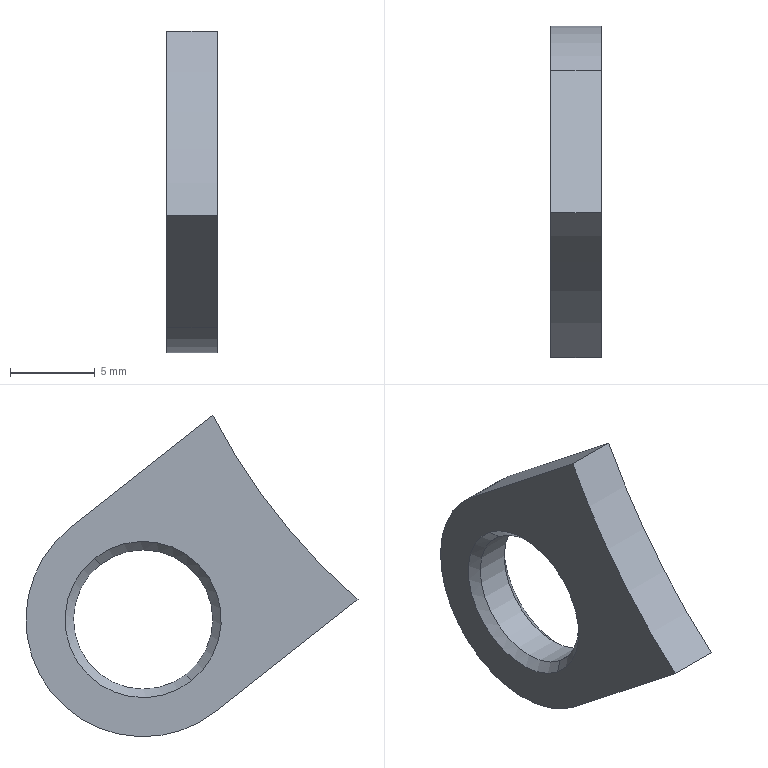Part | SolidWorks | features BaseBody 1 | 1 solid | 12 faces | box 3 x 19.549 x 18.922 mm | volume 482.4 mm3 | cone 4 | cylinder 4 | plane 4 | commonest cylinder face diameters 8.2 x2 13.8 x1 72 x1
STEP:
#1=CARTESIAN_POINT('',(274.5,36.037,-21.279));
#2=VERTEX_POINT('',#1);
#3=CARTESIAN_POINT('',(274.5,30.963,-27.721));
#4=VERTEX_POINT('',#3);
#5=CARTESIAN_POINT('',(274.5,33.5,-24.5));
#6=DIRECTION('',(1.,0.,0.));
#7=DIRECTION('',(0.,-0.6189,-0.7855));
#8=AXIS2_PLACEMENT_3D('',#5,#6,#7);
#9=CIRCLE('',#8,4.1);
#10=EDGE_CURVE('',#2,#4,#9,.T.);
#11=ORIENTED_EDGE('',*,*,#10,.F.);
#12=CARTESIAN_POINT('',(275.,36.347,-20.887));
#13=VERTEX_POINT('',#12);
#14=CARTESIAN_POINT('',(274.5,36.037,-21.279));
#15=DIRECTION('',(0.7071,0.4376,0.5554));
#16=VECTOR('',#15,1000.);
#17=LINE('',#14,#16);
#18=EDGE_CURVE('',#2,#13,#17,.T.);
#19=ORIENTED_EDGE('',*,*,#18,.T.);
#20=CARTESIAN_POINT('',(275.,30.653,-28.113));
#21=VERTEX_POINT('',#20);
#22=CARTESIAN_POINT('',(275.,33.5,-24.5));
#23=DIRECTION('',(-1.,0.,0.));
#24=DIRECTION('',(0.,-0.6189,-0.7855));
#25=AXIS2_PLACEMENT_3D('',#22,#23,#24);
#26=CIRCLE('',#25,4.6);
#27=EDGE_CURVE('',#21,#13,#26,.T.);
#28=ORIENTED_EDGE('',*,*,#27,.F.);
#29=CARTESIAN_POINT('',(274.5,30.963,-27.721));
#30=DIRECTION('',(0.7071,-0.4376,-0.5554));
#31=VECTOR('',#30,1000.);
#32=LINE('',#29,#31);
#33=EDGE_CURVE('',#4,#21,#32,.T.);
#34=ORIENTED_EDGE('',*,*,#33,.F.);
#35=EDGE_LOOP('',(#11,#19,#28,#34));
#36=FACE_OUTER_BOUND('',#35,.T.);
#37=CARTESIAN_POINT('',(274.5,33.5,-24.5));
#38=DIRECTION('',(1.,0.,0.));
#39=DIRECTION('',(0.,-0.6189,-0.7855));
#40=AXIS2_PLACEMENT_3D('',#37,#38,#39);
#41=CONICAL_SURFACE('',#40,4.1,0.7854);
#42=ADVANCED_FACE('',(#36),#41,.F.);
#43=CARTESIAN_POINT('',(272.5,30.963,-27.721));
#44=VERTEX_POINT('',#43);
#45=CARTESIAN_POINT('',(272.5,36.037,-21.279));
#46=VERTEX_POINT('',#45);
#47=CARTESIAN_POINT('',(272.5,33.5,-24.5));
#48=DIRECTION('',(-1.,0.,0.));
#49=DIRECTION('',(0.,-0.6189,-0.7855));
#50=AXIS2_PLACEMENT_3D('',#47,#48,#49);
#51=CIRCLE('',#50,4.1);
#52=EDGE_CURVE('',#44,#46,#51,.T.);
#53=ORIENTED_EDGE('',*,*,#52,.F.);
#54=CARTESIAN_POINT('',(272.,30.653,-28.113));
#55=VERTEX_POINT('',#54);
#56=CARTESIAN_POINT('',(272.,30.653,-28.113));
#57=DIRECTION('',(-0.7071,-0.4376,-0.5554));
#58=VECTOR('',#57,1000.);
#59=LINE('',#56,#58);
#60=EDGE_CURVE('',#44,#55,#59,.T.);
#61=ORIENTED_EDGE('',*,*,#60,.T.);
#62=CARTESIAN_POINT('',(272.,36.347,-20.887));
#63=VERTEX_POINT('',#62);
#64=CARTESIAN_POINT('',(272.,33.5,-24.5));
#65=DIRECTION('',(1.,0.,0.));
#66=DIRECTION('',(0.,-0.6189,-0.7855));
#67=AXIS2_PLACEMENT_3D('',#64,#65,#66);
#68=CIRCLE('',#67,4.6);
#69=EDGE_CURVE('',#63,#55,#68,.T.);
#70=ORIENTED_EDGE('',*,*,#69,.F.);
#71=CARTESIAN_POINT('',(272.,36.347,-20.887));
#72=DIRECTION('',(-0.7071,0.4376,0.5554));
#73=VECTOR('',#72,1000.);
#74=LINE('',#71,#73);
#75=EDGE_CURVE('',#46,#63,#74,.T.);
#76=ORIENTED_EDGE('',*,*,#75,.F.);
#77=EDGE_LOOP('',(#53,#61,#70,#76));
#78=FACE_OUTER_BOUND('',#77,.T.);
#79=CARTESIAN_POINT('',(272.,33.5,-24.5));
#80=DIRECTION('',(-1.,0.,0.));
#81=DIRECTION('',(0.,0.6189,0.7855));
#82=AXIS2_PLACEMENT_3D('',#79,#80,#81);
#83=CONICAL_SURFACE('',#82,4.6,0.7854);
#84=ADVANCED_FACE('',(#78),#83,.F.);
#85=ORIENTED_EDGE('',*,*,#10,.T.);
#86=CARTESIAN_POINT('',(275.,30.963,-27.721));
#87=DIRECTION('',(-1.,0.,0.));
#88=VECTOR('',#87,1000.);
#89=LINE('',#86,#88);
#90=EDGE_CURVE('',#4,#44,#89,.T.);
#91=ORIENTED_EDGE('',*,*,#90,.T.);
#92=ORIENTED_EDGE('',*,*,#52,.T.);
#93=CARTESIAN_POINT('',(275.,36.037,-21.279));
#94=DIRECTION('',(-1.,0.,0.));
#95=VECTOR('',#94,1000.);
#96=LINE('',#93,#95);
#97=EDGE_CURVE('',#2,#46,#96,.T.);
#98=ORIENTED_EDGE('',*,*,#97,.F.);
#99=EDGE_LOOP('',(#85,#91,#92,#98));
#100=FACE_OUTER_BOUND('',#99,.T.);
#101=CARTESIAN_POINT('',(275.,33.5,-24.5));
#102=DIRECTION('',(-1.,0.,0.));
#103=DIRECTION('',(0.,0.6189,0.7855));
#104=AXIS2_PLACEMENT_3D('',#101,#102,#103);
#105=CYLINDRICAL_SURFACE('',#104,4.1);
#106=ADVANCED_FACE('',(#100),#105,.F.);
#107=ORIENTED_EDGE('',*,*,#27,.T.);
#108=CARTESIAN_POINT('',(275.,33.5,-24.5));
#109=DIRECTION('',(-1.,0.,0.));
#110=DIRECTION('',(0.,-0.6189,-0.7855));
#111=AXIS2_PLACEMENT_3D('',#108,#109,#110);
#112=CIRCLE('',#111,4.6);
#113=EDGE_CURVE('',#13,#21,#112,.T.);
#114=ORIENTED_EDGE('',*,*,#113,.T.);
#115=EDGE_LOOP('',(#107,#114));
#116=FACE_BOUND('',#115,.T.);
#117=CARTESIAN_POINT('',(275.,29.23,-29.92));
#118=VERTEX_POINT('',#117);
#119=CARTESIAN_POINT('',(275.,37.77,-19.08));
#120=VERTEX_POINT('',#119);
#121=CARTESIAN_POINT('',(275.,33.5,-24.5));
#122=DIRECTION('',(1.,0.,0.));
#123=DIRECTION('',(0.,-0.6189,-0.7855));
#124=AXIS2_PLACEMENT_3D('',#121,#122,#123);
#125=CIRCLE('',#124,6.9);
#126=EDGE_CURVE('',#118,#120,#125,.T.);
#127=ORIENTED_EDGE('',*,*,#126,.T.);
#128=CARTESIAN_POINT('',(275.,29.391,-12.478));
#129=VERTEX_POINT('',#128);
#130=CARTESIAN_POINT('',(275.,37.77,-19.08));
#131=DIRECTION('',(0.,-0.7855,0.6189));
#132=VECTOR('',#131,1000.);
#133=LINE('',#130,#132);
#134=EDGE_CURVE('',#120,#129,#133,.T.);
#135=ORIENTED_EDGE('',*,*,#134,.T.);
#136=CARTESIAN_POINT('',(275.,20.851,-23.318));
#137=VERTEX_POINT('',#136);
#138=CARTESIAN_POINT('',(275.,-2.633,3.967));
#139=DIRECTION('',(-1.,0.,0.));
#140=DIRECTION('',(0.,-0.6189,-0.7855));
#141=AXIS2_PLACEMENT_3D('',#138,#139,#140);
#142=CIRCLE('',#141,36.);
#143=EDGE_CURVE('',#129,#137,#142,.T.);
#144=ORIENTED_EDGE('',*,*,#143,.T.);
#145=CARTESIAN_POINT('',(275.,29.23,-29.92));
#146=DIRECTION('',(0.,0.7855,-0.6189));
#147=VECTOR('',#146,1000.);
#148=LINE('',#145,#147);
#149=EDGE_CURVE('',#137,#118,#148,.T.);
#150=ORIENTED_EDGE('',*,*,#149,.T.);
#151=EDGE_LOOP('',(#127,#135,#144,#150));
#152=FACE_OUTER_BOUND('',#151,.T.);
#153=CARTESIAN_POINT('',(275.,33.5,-24.5));
#154=DIRECTION('',(1.,0.,0.));
#155=DIRECTION('',(0.,-0.6189,-0.7855));
#156=AXIS2_PLACEMENT_3D('',#153,#154,#155);
#157=PLANE('',#156);
#158=ADVANCED_FACE('',(#116,#152),#157,.T.);
#159=ORIENTED_EDGE('',*,*,#69,.T.);
#160=CARTESIAN_POINT('',(272.,33.5,-24.5));
#161=DIRECTION('',(1.,0.,0.));
#162=DIRECTION('',(0.,-0.6189,-0.7855));
#163=AXIS2_PLACEMENT_3D('',#160,#161,#162);
#164=CIRCLE('',#163,4.6);
#165=EDGE_CURVE('',#55,#63,#164,.T.);
#166=ORIENTED_EDGE('',*,*,#165,.T.);
#167=EDGE_LOOP('',(#159,#166));
#168=FACE_BOUND('',#167,.T.);
#169=CARTESIAN_POINT('',(272.,29.23,-29.92));
#170=VERTEX_POINT('',#169);
#171=CARTESIAN_POINT('',(272.,37.77,-19.08));
#172=VERTEX_POINT('',#171);
#173=CARTESIAN_POINT('',(272.,33.5,-24.5));
#174=DIRECTION('',(1.,0.,0.));
#175=DIRECTION('',(0.,-0.6189,-0.7855));
#176=AXIS2_PLACEMENT_3D('',#173,#174,#175);
#177=CIRCLE('',#176,6.9);
#178=EDGE_CURVE('',#170,#172,#177,.T.);
#179=ORIENTED_EDGE('',*,*,#178,.F.);
#180=CARTESIAN_POINT('',(272.,20.851,-23.318));
#181=VERTEX_POINT('',#180);
#182=CARTESIAN_POINT('',(272.,29.23,-29.92));
#183=DIRECTION('',(0.,0.7855,-0.6189));
#184=VECTOR('',#183,1000.);
#185=LINE('',#182,#184);
#186=EDGE_CURVE('',#181,#170,#185,.T.);
#187=ORIENTED_EDGE('',*,*,#186,.F.);
#188=CARTESIAN_POINT('',(272.,29.391,-12.478));
#189=VERTEX_POINT('',#188);
#190=CARTESIAN_POINT('',(272.,-2.633,3.967));
#191=DIRECTION('',(-1.,0.,0.));
#192=DIRECTION('',(0.,-0.6189,-0.7855));
#193=AXIS2_PLACEMENT_3D('',#190,#191,#192);
#194=CIRCLE('',#193,36.);
#195=EDGE_CURVE('',#189,#181,#194,.T.);
#196=ORIENTED_EDGE('',*,*,#195,.F.);
#197=CARTESIAN_POINT('',(272.,37.77,-19.08));
#198=DIRECTION('',(0.,-0.7855,0.6189));
#199=VECTOR('',#198,1000.);
#200=LINE('',#197,#199);
#201=EDGE_CURVE('',#172,#189,#200,.T.);
#202=ORIENTED_EDGE('',*,*,#201,.F.);
#203=EDGE_LOOP('',(#179,#187,#196,#202));
#204=FACE_OUTER_BOUND('',#203,.T.);
#205=CARTESIAN_POINT('',(272.,33.5,-24.5));
#206=DIRECTION('',(1.,0.,0.));
#207=DIRECTION('',(0.,-0.6189,-0.7855));
#208=AXIS2_PLACEMENT_3D('',#205,#206,#207);
#209=PLANE('',#208);
#210=ADVANCED_FACE('',(#168,#204),#209,.F.);
#211=ORIENTED_EDGE('',*,*,#178,.T.);
#212=CARTESIAN_POINT('',(275.,37.77,-19.08));
#213=DIRECTION('',(-1.,0.,0.));
#214=VECTOR('',#213,1000.);
#215=LINE('',#212,#214);
#216=EDGE_CURVE('',#120,#172,#215,.T.);
#217=ORIENTED_EDGE('',*,*,#216,.F.);
#218=ORIENTED_EDGE('',*,*,#126,.F.);
#219=CARTESIAN_POINT('',(275.,29.23,-29.92));
#220=DIRECTION('',(-1.,0.,0.));
#221=VECTOR('',#220,1000.);
#222=LINE('',#219,#221);
#223=EDGE_CURVE('',#118,#170,#222,.T.);
#224=ORIENTED_EDGE('',*,*,#223,.T.);
#225=EDGE_LOOP('',(#211,#217,#218,#224));
#226=FACE_OUTER_BOUND('',#225,.T.);
#227=CARTESIAN_POINT('',(275.,33.5,-24.5));
#228=DIRECTION('',(-1.,0.,0.));
#229=DIRECTION('',(0.,0.6189,0.7855));
#230=AXIS2_PLACEMENT_3D('',#227,#228,#229);
#231=CYLINDRICAL_SURFACE('',#230,6.9);
#232=ADVANCED_FACE('',(#226),#231,.T.);
#233=ORIENTED_EDGE('',*,*,#201,.T.);
#234=CARTESIAN_POINT('',(275.,29.391,-12.478));
#235=DIRECTION('',(-1.,0.,0.));
#236=VECTOR('',#235,1000.);
#237=LINE('',#234,#236);
#238=EDGE_CURVE('',#129,#189,#237,.T.);
#239=ORIENTED_EDGE('',*,*,#238,.F.);
#240=ORIENTED_EDGE('',*,*,#134,.F.);
#241=ORIENTED_EDGE('',*,*,#216,.T.);
#242=EDGE_LOOP('',(#233,#239,#240,#241));
#243=FACE_OUTER_BOUND('',#242,.T.);
#244=CARTESIAN_POINT('',(275.,37.77,-19.08));
#245=DIRECTION('',(0.,-0.6189,-0.7855));
#246=DIRECTION('',(0.,0.7855,-0.6189));
#247=AXIS2_PLACEMENT_3D('',#244,#245,#246);
#248=PLANE('',#247);
#249=ADVANCED_FACE('',(#243),#248,.F.);
#250=ORIENTED_EDGE('',*,*,#195,.T.);
#251=CARTESIAN_POINT('',(275.,20.851,-23.318));
#252=DIRECTION('',(-1.,0.,0.));
#253=VECTOR('',#252,1000.);
#254=LINE('',#251,#253);
#255=EDGE_CURVE('',#137,#181,#254,.T.);
#256=ORIENTED_EDGE('',*,*,#255,.F.);
#257=ORIENTED_EDGE('',*,*,#143,.F.);
#258=ORIENTED_EDGE('',*,*,#238,.T.);
#259=EDGE_LOOP('',(#250,#256,#257,#258));
#260=FACE_OUTER_BOUND('',#259,.T.);
#261=CARTESIAN_POINT('',(275.,-2.633,3.967));
#262=DIRECTION('',(-1.,0.,0.));
#263=DIRECTION('',(0.,0.6189,0.7855));
#264=AXIS2_PLACEMENT_3D('',#261,#262,#263);
#265=CYLINDRICAL_SURFACE('',#264,36.);
#266=ADVANCED_FACE('',(#260),#265,.F.);
#267=ORIENTED_EDGE('',*,*,#186,.T.);
#268=ORIENTED_EDGE('',*,*,#223,.F.);
#269=ORIENTED_EDGE('',*,*,#149,.F.);
#270=ORIENTED_EDGE('',*,*,#255,.T.);
#271=EDGE_LOOP('',(#267,#268,#269,#270));
#272=FACE_OUTER_BOUND('',#271,.T.);
#273=CARTESIAN_POINT('',(275.,29.23,-29.92));
#274=DIRECTION('',(0.,0.6189,0.7855));
#275=DIRECTION('',(0.,-0.7855,0.6189));
#276=AXIS2_PLACEMENT_3D('',#273,#274,#275);
#277=PLANE('',#276);
#278=ADVANCED_FACE('',(#272),#277,.F.);
#279=ORIENTED_EDGE('',*,*,#90,.F.);
#280=CARTESIAN_POINT('',(274.5,33.5,-24.5));
#281=DIRECTION('',(1.,0.,0.));
#282=DIRECTION('',(0.,-0.6189,-0.7855));
#283=AXIS2_PLACEMENT_3D('',#280,#281,#282);
#284=CIRCLE('',#283,4.1);
#285=EDGE_CURVE('',#4,#2,#284,.T.);
#286=ORIENTED_EDGE('',*,*,#285,.T.);
#287=ORIENTED_EDGE('',*,*,#97,.T.);
#288=CARTESIAN_POINT('',(272.5,33.5,-24.5));
#289=DIRECTION('',(-1.,0.,0.));
#290=DIRECTION('',(0.,-0.6189,-0.7855));
#291=AXIS2_PLACEMENT_3D('',#288,#289,#290);
#292=CIRCLE('',#291,4.1);
#293=EDGE_CURVE('',#46,#44,#292,.T.);
#294=ORIENTED_EDGE('',*,*,#293,.T.);
#295=EDGE_LOOP('',(#279,#286,#287,#294));
#296=FACE_OUTER_BOUND('',#295,.T.);
#297=CARTESIAN_POINT('',(275.,33.5,-24.5));
#298=DIRECTION('',(-1.,0.,0.));
#299=DIRECTION('',(0.,0.6189,0.7855));
#300=AXIS2_PLACEMENT_3D('',#297,#298,#299);
#301=CYLINDRICAL_SURFACE('',#300,4.1);
#302=ADVANCED_FACE('',(#296),#301,.F.);
#303=ORIENTED_EDGE('',*,*,#60,.F.);
#304=ORIENTED_EDGE('',*,*,#293,.F.);
#305=ORIENTED_EDGE('',*,*,#75,.T.);
#306=ORIENTED_EDGE('',*,*,#165,.F.);
#307=EDGE_LOOP('',(#303,#304,#305,#306));
#308=FACE_OUTER_BOUND('',#307,.T.);
#309=CARTESIAN_POINT('',(272.,33.5,-24.5));
#310=DIRECTION('',(-1.,0.,0.));
#311=DIRECTION('',(0.,0.6189,0.7855));
#312=AXIS2_PLACEMENT_3D('',#309,#310,#311);
#313=CONICAL_SURFACE('',#312,4.6,0.7854);
#314=ADVANCED_FACE('',(#308),#313,.F.);
#315=ORIENTED_EDGE('',*,*,#18,.F.);
#316=ORIENTED_EDGE('',*,*,#285,.F.);
#317=ORIENTED_EDGE('',*,*,#33,.T.);
#318=ORIENTED_EDGE('',*,*,#113,.F.);
#319=EDGE_LOOP('',(#315,#316,#317,#318));
#320=FACE_OUTER_BOUND('',#319,.T.);
#321=CARTESIAN_POINT('',(274.5,33.5,-24.5));
#322=DIRECTION('',(1.,0.,0.));
#323=DIRECTION('',(0.,-0.6189,-0.7855));
#324=AXIS2_PLACEMENT_3D('',#321,#322,#323);
#325=CONICAL_SURFACE('',#324,4.1,0.7854);
#326=ADVANCED_FACE('',(#320),#325,.F.);
#327=CLOSED_SHELL('',(#42,#84,#106,#158,#210,#232,#249,#266,#278,#302,#314,#326));
#328=MANIFOLD_SOLID_BREP('',#327);
#329=CARTESIAN_POINT('',(0.,0.,0.));
#330=DIRECTION('',(0.,0.,1.));
#331=DIRECTION('',(1.,0.,0.));
#332=AXIS2_PLACEMENT_3D('',#329,#330,#331);
#333=(LENGTH_UNIT()NAMED_UNIT(*)SI_UNIT(.MILLI.,.METRE.));
#334=UNCERTAINTY_MEASURE_WITH_UNIT(LENGTH_MEASURE(0.00001),#333,'','');
#335=(NAMED_UNIT(*)PLANE_ANGLE_UNIT()SI_UNIT($,.RADIAN.));
#336=(NAMED_UNIT(*)SI_UNIT($,.STERADIAN.)SOLID_ANGLE_UNIT());
#337=(GEOMETRIC_REPRESENTATION_CONTEXT(3)GLOBAL_UNCERTAINTY_ASSIGNED_CONTEXT((#334))GLOBAL_UNIT_ASSIGNED_CONTEXT((#333,#335,#336))REPRESENTATION_CONTEXT('',''));
#338=ADVANCED_BREP_SHAPE_REPRESENTATION('',(#328,#332),#337);